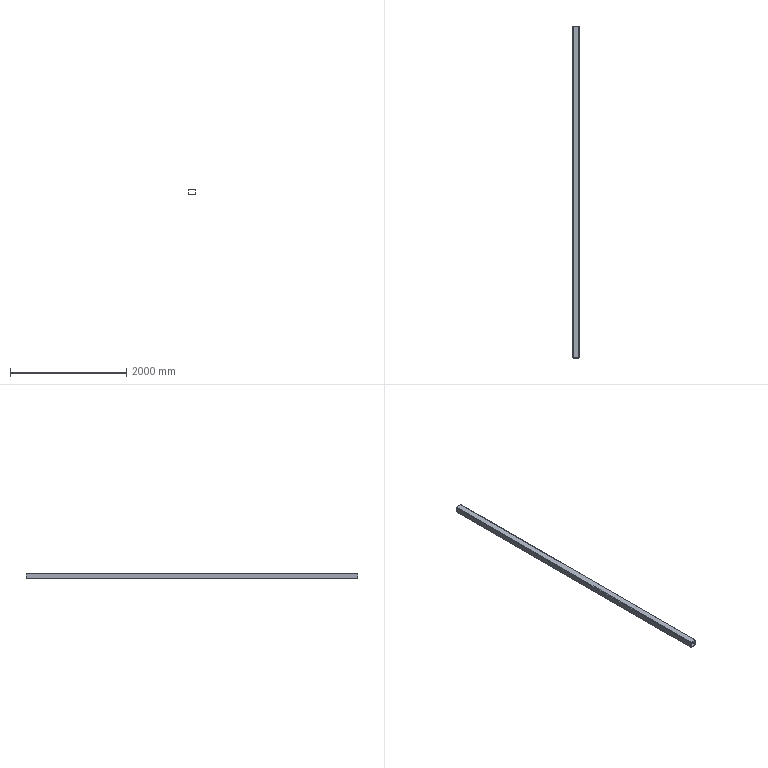Part | SolidWorks | features ExtruThin 1 | 1 solid | 18 faces | box 120 x 5702 x 100 mm | volume 9357335 mm3 | plane 10 | cylinder 8 | commonest cylinder face diameters 12 x4 20 x4
STEP:
#1=CARTESIAN_POINT('',(60.,2851.,-40.));
#2=VERTEX_POINT('',#1);
#3=CARTESIAN_POINT('',(50.,2851.,-50.));
#4=VERTEX_POINT('',#3);
#5=CARTESIAN_POINT('',(50.,2851.,-40.));
#6=DIRECTION('',(0.,1.,0.));
#7=DIRECTION('',(0.,0.,-1.));
#8=AXIS2_PLACEMENT_3D('',#5,#6,#7);
#9=CIRCLE('',#8,10.);
#10=EDGE_CURVE('',#2,#4,#9,.T.);
#11=ORIENTED_EDGE('',*,*,#10,.T.);
#12=CARTESIAN_POINT('',(-50.,2851.,-50.));
#13=VERTEX_POINT('',#12);
#14=CARTESIAN_POINT('',(-50.,2851.,-50.));
#15=DIRECTION('',(-1.,0.,0.));
#16=VECTOR('',#15,1000.);
#17=LINE('',#14,#16);
#18=EDGE_CURVE('',#4,#13,#17,.T.);
#19=ORIENTED_EDGE('',*,*,#18,.T.);
#20=CARTESIAN_POINT('',(-60.,2851.,-40.));
#21=VERTEX_POINT('',#20);
#22=CARTESIAN_POINT('',(-50.,2851.,-40.));
#23=DIRECTION('',(0.,1.,0.));
#24=DIRECTION('',(0.,0.,1.));
#25=AXIS2_PLACEMENT_3D('',#22,#23,#24);
#26=CIRCLE('',#25,10.);
#27=EDGE_CURVE('',#13,#21,#26,.T.);
#28=ORIENTED_EDGE('',*,*,#27,.T.);
#29=CARTESIAN_POINT('',(-60.,2851.,40.));
#30=VERTEX_POINT('',#29);
#31=CARTESIAN_POINT('',(-60.,2851.,-40.));
#32=DIRECTION('',(0.,0.,1.));
#33=VECTOR('',#32,1000.);
#34=LINE('',#31,#33);
#35=EDGE_CURVE('',#21,#30,#34,.T.);
#36=ORIENTED_EDGE('',*,*,#35,.T.);
#37=CARTESIAN_POINT('',(-50.,2851.,50.));
#38=VERTEX_POINT('',#37);
#39=CARTESIAN_POINT('',(-50.,2851.,40.));
#40=DIRECTION('',(0.,1.,0.));
#41=DIRECTION('',(0.,0.,1.));
#42=AXIS2_PLACEMENT_3D('',#39,#40,#41);
#43=CIRCLE('',#42,10.);
#44=EDGE_CURVE('',#30,#38,#43,.T.);
#45=ORIENTED_EDGE('',*,*,#44,.T.);
#46=CARTESIAN_POINT('',(50.,2851.,50.));
#47=VERTEX_POINT('',#46);
#48=CARTESIAN_POINT('',(-50.,2851.,50.));
#49=DIRECTION('',(1.,0.,0.));
#50=VECTOR('',#49,1000.);
#51=LINE('',#48,#50);
#52=EDGE_CURVE('',#38,#47,#51,.T.);
#53=ORIENTED_EDGE('',*,*,#52,.T.);
#54=CARTESIAN_POINT('',(60.,2851.,40.));
#55=VERTEX_POINT('',#54);
#56=CARTESIAN_POINT('',(50.,2851.,40.));
#57=DIRECTION('',(0.,1.,0.));
#58=DIRECTION('',(0.,0.,1.));
#59=AXIS2_PLACEMENT_3D('',#56,#57,#58);
#60=CIRCLE('',#59,10.);
#61=EDGE_CURVE('',#47,#55,#60,.T.);
#62=ORIENTED_EDGE('',*,*,#61,.T.);
#63=CARTESIAN_POINT('',(60.,2851.,-40.));
#64=DIRECTION('',(0.,0.,-1.));
#65=VECTOR('',#64,1000.);
#66=LINE('',#63,#65);
#67=EDGE_CURVE('',#55,#2,#66,.T.);
#68=ORIENTED_EDGE('',*,*,#67,.T.);
#69=EDGE_LOOP('',(#11,#19,#28,#36,#45,#53,#62,#68));
#70=FACE_OUTER_BOUND('',#69,.T.);
#71=CARTESIAN_POINT('',(50.,2851.,-46.));
#72=VERTEX_POINT('',#71);
#73=CARTESIAN_POINT('',(-50.,2851.,-46.));
#74=VERTEX_POINT('',#73);
#75=CARTESIAN_POINT('',(50.,2851.,-46.));
#76=DIRECTION('',(-1.,0.,0.));
#77=VECTOR('',#76,1000.);
#78=LINE('',#75,#77);
#79=EDGE_CURVE('',#72,#74,#78,.T.);
#80=ORIENTED_EDGE('',*,*,#79,.F.);
#81=CARTESIAN_POINT('',(56.,2851.,-40.));
#82=VERTEX_POINT('',#81);
#83=CARTESIAN_POINT('',(50.,2851.,-40.));
#84=DIRECTION('',(0.,1.,0.));
#85=DIRECTION('',(-1.,0.,0.));
#86=AXIS2_PLACEMENT_3D('',#83,#84,#85);
#87=CIRCLE('',#86,6.);
#88=EDGE_CURVE('',#82,#72,#87,.T.);
#89=ORIENTED_EDGE('',*,*,#88,.F.);
#90=CARTESIAN_POINT('',(56.,2851.,40.));
#91=VERTEX_POINT('',#90);
#92=CARTESIAN_POINT('',(56.,2851.,-40.));
#93=DIRECTION('',(0.,0.,-1.));
#94=VECTOR('',#93,1000.);
#95=LINE('',#92,#94);
#96=EDGE_CURVE('',#91,#82,#95,.T.);
#97=ORIENTED_EDGE('',*,*,#96,.F.);
#98=CARTESIAN_POINT('',(50.,2851.,46.));
#99=VERTEX_POINT('',#98);
#100=CARTESIAN_POINT('',(50.,2851.,40.));
#101=DIRECTION('',(0.,1.,0.));
#102=DIRECTION('',(-1.,0.,0.));
#103=AXIS2_PLACEMENT_3D('',#100,#101,#102);
#104=CIRCLE('',#103,6.);
#105=EDGE_CURVE('',#99,#91,#104,.T.);
#106=ORIENTED_EDGE('',*,*,#105,.F.);
#107=CARTESIAN_POINT('',(-50.,2851.,46.));
#108=VERTEX_POINT('',#107);
#109=CARTESIAN_POINT('',(50.,2851.,46.));
#110=DIRECTION('',(1.,0.,0.));
#111=VECTOR('',#110,1000.);
#112=LINE('',#109,#111);
#113=EDGE_CURVE('',#108,#99,#112,.T.);
#114=ORIENTED_EDGE('',*,*,#113,.F.);
#115=CARTESIAN_POINT('',(-56.,2851.,40.));
#116=VERTEX_POINT('',#115);
#117=CARTESIAN_POINT('',(-50.,2851.,40.));
#118=DIRECTION('',(0.,1.,0.));
#119=DIRECTION('',(-1.,0.,0.));
#120=AXIS2_PLACEMENT_3D('',#117,#118,#119);
#121=CIRCLE('',#120,6.);
#122=EDGE_CURVE('',#116,#108,#121,.T.);
#123=ORIENTED_EDGE('',*,*,#122,.F.);
#124=CARTESIAN_POINT('',(-56.,2851.,-40.));
#125=VERTEX_POINT('',#124);
#126=CARTESIAN_POINT('',(-56.,2851.,-40.));
#127=DIRECTION('',(0.,0.,1.));
#128=VECTOR('',#127,1000.);
#129=LINE('',#126,#128);
#130=EDGE_CURVE('',#125,#116,#129,.T.);
#131=ORIENTED_EDGE('',*,*,#130,.F.);
#132=CARTESIAN_POINT('',(-50.,2851.,-40.));
#133=DIRECTION('',(0.,1.,0.));
#134=DIRECTION('',(-1.,0.,0.));
#135=AXIS2_PLACEMENT_3D('',#132,#133,#134);
#136=CIRCLE('',#135,6.);
#137=EDGE_CURVE('',#74,#125,#136,.T.);
#138=ORIENTED_EDGE('',*,*,#137,.F.);
#139=EDGE_LOOP('',(#80,#89,#97,#106,#114,#123,#131,#138));
#140=FACE_BOUND('',#139,.T.);
#141=CARTESIAN_POINT('',(50.,2851.,-40.));
#142=DIRECTION('',(0.,1.,0.));
#143=DIRECTION('',(0.,0.,1.));
#144=AXIS2_PLACEMENT_3D('',#141,#142,#143);
#145=PLANE('',#144);
#146=ADVANCED_FACE('',(#70,#140),#145,.T.);
#147=CARTESIAN_POINT('',(60.,-2851.,-40.));
#148=VERTEX_POINT('',#147);
#149=CARTESIAN_POINT('',(50.,-2851.,-50.));
#150=VERTEX_POINT('',#149);
#151=CARTESIAN_POINT('',(50.,-2851.,-40.));
#152=DIRECTION('',(0.,1.,0.));
#153=DIRECTION('',(0.,0.,-1.));
#154=AXIS2_PLACEMENT_3D('',#151,#152,#153);
#155=CIRCLE('',#154,10.);
#156=EDGE_CURVE('',#148,#150,#155,.T.);
#157=ORIENTED_EDGE('',*,*,#156,.F.);
#158=CARTESIAN_POINT('',(60.,-2851.,40.));
#159=VERTEX_POINT('',#158);
#160=CARTESIAN_POINT('',(60.,-2851.,-40.));
#161=DIRECTION('',(0.,0.,-1.));
#162=VECTOR('',#161,1000.);
#163=LINE('',#160,#162);
#164=EDGE_CURVE('',#159,#148,#163,.T.);
#165=ORIENTED_EDGE('',*,*,#164,.F.);
#166=CARTESIAN_POINT('',(50.,-2851.,50.));
#167=VERTEX_POINT('',#166);
#168=CARTESIAN_POINT('',(50.,-2851.,40.));
#169=DIRECTION('',(0.,1.,0.));
#170=DIRECTION('',(0.,0.,1.));
#171=AXIS2_PLACEMENT_3D('',#168,#169,#170);
#172=CIRCLE('',#171,10.);
#173=EDGE_CURVE('',#167,#159,#172,.T.);
#174=ORIENTED_EDGE('',*,*,#173,.F.);
#175=CARTESIAN_POINT('',(-50.,-2851.,50.));
#176=VERTEX_POINT('',#175);
#177=CARTESIAN_POINT('',(-50.,-2851.,50.));
#178=DIRECTION('',(1.,0.,0.));
#179=VECTOR('',#178,1000.);
#180=LINE('',#177,#179);
#181=EDGE_CURVE('',#176,#167,#180,.T.);
#182=ORIENTED_EDGE('',*,*,#181,.F.);
#183=CARTESIAN_POINT('',(-60.,-2851.,40.));
#184=VERTEX_POINT('',#183);
#185=CARTESIAN_POINT('',(-50.,-2851.,40.));
#186=DIRECTION('',(0.,1.,0.));
#187=DIRECTION('',(0.,0.,1.));
#188=AXIS2_PLACEMENT_3D('',#185,#186,#187);
#189=CIRCLE('',#188,10.);
#190=EDGE_CURVE('',#184,#176,#189,.T.);
#191=ORIENTED_EDGE('',*,*,#190,.F.);
#192=CARTESIAN_POINT('',(-60.,-2851.,-40.));
#193=VERTEX_POINT('',#192);
#194=CARTESIAN_POINT('',(-60.,-2851.,-40.));
#195=DIRECTION('',(0.,0.,1.));
#196=VECTOR('',#195,1000.);
#197=LINE('',#194,#196);
#198=EDGE_CURVE('',#193,#184,#197,.T.);
#199=ORIENTED_EDGE('',*,*,#198,.F.);
#200=CARTESIAN_POINT('',(-50.,-2851.,-50.));
#201=VERTEX_POINT('',#200);
#202=CARTESIAN_POINT('',(-50.,-2851.,-40.));
#203=DIRECTION('',(0.,1.,0.));
#204=DIRECTION('',(0.,0.,1.));
#205=AXIS2_PLACEMENT_3D('',#202,#203,#204);
#206=CIRCLE('',#205,10.);
#207=EDGE_CURVE('',#201,#193,#206,.T.);
#208=ORIENTED_EDGE('',*,*,#207,.F.);
#209=CARTESIAN_POINT('',(-50.,-2851.,-50.));
#210=DIRECTION('',(-1.,0.,0.));
#211=VECTOR('',#210,1000.);
#212=LINE('',#209,#211);
#213=EDGE_CURVE('',#150,#201,#212,.T.);
#214=ORIENTED_EDGE('',*,*,#213,.F.);
#215=EDGE_LOOP('',(#157,#165,#174,#182,#191,#199,#208,#214));
#216=FACE_OUTER_BOUND('',#215,.T.);
#217=CARTESIAN_POINT('',(56.,-2851.,-40.));
#218=VERTEX_POINT('',#217);
#219=CARTESIAN_POINT('',(50.,-2851.,-46.));
#220=VERTEX_POINT('',#219);
#221=CARTESIAN_POINT('',(50.,-2851.,-40.));
#222=DIRECTION('',(0.,1.,0.));
#223=DIRECTION('',(-1.,0.,0.));
#224=AXIS2_PLACEMENT_3D('',#221,#222,#223);
#225=CIRCLE('',#224,6.);
#226=EDGE_CURVE('',#218,#220,#225,.T.);
#227=ORIENTED_EDGE('',*,*,#226,.T.);
#228=CARTESIAN_POINT('',(-50.,-2851.,-46.));
#229=VERTEX_POINT('',#228);
#230=CARTESIAN_POINT('',(50.,-2851.,-46.));
#231=DIRECTION('',(-1.,0.,0.));
#232=VECTOR('',#231,1000.);
#233=LINE('',#230,#232);
#234=EDGE_CURVE('',#220,#229,#233,.T.);
#235=ORIENTED_EDGE('',*,*,#234,.T.);
#236=CARTESIAN_POINT('',(-56.,-2851.,-40.));
#237=VERTEX_POINT('',#236);
#238=CARTESIAN_POINT('',(-50.,-2851.,-40.));
#239=DIRECTION('',(0.,1.,0.));
#240=DIRECTION('',(-1.,0.,0.));
#241=AXIS2_PLACEMENT_3D('',#238,#239,#240);
#242=CIRCLE('',#241,6.);
#243=EDGE_CURVE('',#229,#237,#242,.T.);
#244=ORIENTED_EDGE('',*,*,#243,.T.);
#245=CARTESIAN_POINT('',(-56.,-2851.,40.));
#246=VERTEX_POINT('',#245);
#247=CARTESIAN_POINT('',(-56.,-2851.,-40.));
#248=DIRECTION('',(0.,0.,1.));
#249=VECTOR('',#248,1000.);
#250=LINE('',#247,#249);
#251=EDGE_CURVE('',#237,#246,#250,.T.);
#252=ORIENTED_EDGE('',*,*,#251,.T.);
#253=CARTESIAN_POINT('',(-50.,-2851.,46.));
#254=VERTEX_POINT('',#253);
#255=CARTESIAN_POINT('',(-50.,-2851.,40.));
#256=DIRECTION('',(0.,1.,0.));
#257=DIRECTION('',(-1.,0.,0.));
#258=AXIS2_PLACEMENT_3D('',#255,#256,#257);
#259=CIRCLE('',#258,6.);
#260=EDGE_CURVE('',#246,#254,#259,.T.);
#261=ORIENTED_EDGE('',*,*,#260,.T.);
#262=CARTESIAN_POINT('',(50.,-2851.,46.));
#263=VERTEX_POINT('',#262);
#264=CARTESIAN_POINT('',(50.,-2851.,46.));
#265=DIRECTION('',(1.,0.,0.));
#266=VECTOR('',#265,1000.);
#267=LINE('',#264,#266);
#268=EDGE_CURVE('',#254,#263,#267,.T.);
#269=ORIENTED_EDGE('',*,*,#268,.T.);
#270=CARTESIAN_POINT('',(56.,-2851.,40.));
#271=VERTEX_POINT('',#270);
#272=CARTESIAN_POINT('',(50.,-2851.,40.));
#273=DIRECTION('',(0.,1.,0.));
#274=DIRECTION('',(-1.,0.,0.));
#275=AXIS2_PLACEMENT_3D('',#272,#273,#274);
#276=CIRCLE('',#275,6.);
#277=EDGE_CURVE('',#263,#271,#276,.T.);
#278=ORIENTED_EDGE('',*,*,#277,.T.);
#279=CARTESIAN_POINT('',(56.,-2851.,-40.));
#280=DIRECTION('',(0.,0.,-1.));
#281=VECTOR('',#280,1000.);
#282=LINE('',#279,#281);
#283=EDGE_CURVE('',#271,#218,#282,.T.);
#284=ORIENTED_EDGE('',*,*,#283,.T.);
#285=EDGE_LOOP('',(#227,#235,#244,#252,#261,#269,#278,#284));
#286=FACE_BOUND('',#285,.T.);
#287=CARTESIAN_POINT('',(50.,-2851.,-40.));
#288=DIRECTION('',(0.,1.,0.));
#289=DIRECTION('',(0.,0.,1.));
#290=AXIS2_PLACEMENT_3D('',#287,#288,#289);
#291=PLANE('',#290);
#292=ADVANCED_FACE('',(#216,#286),#291,.F.);
#293=ORIENTED_EDGE('',*,*,#156,.T.);
#294=CARTESIAN_POINT('',(50.,2851.,-50.));
#295=DIRECTION('',(0.,-1.,0.));
#296=VECTOR('',#295,1000.);
#297=LINE('',#294,#296);
#298=EDGE_CURVE('',#4,#150,#297,.T.);
#299=ORIENTED_EDGE('',*,*,#298,.F.);
#300=ORIENTED_EDGE('',*,*,#10,.F.);
#301=CARTESIAN_POINT('',(60.,2851.,-40.));
#302=DIRECTION('',(0.,-1.,0.));
#303=VECTOR('',#302,1000.);
#304=LINE('',#301,#303);
#305=EDGE_CURVE('',#2,#148,#304,.T.);
#306=ORIENTED_EDGE('',*,*,#305,.T.);
#307=EDGE_LOOP('',(#293,#299,#300,#306));
#308=FACE_OUTER_BOUND('',#307,.T.);
#309=CARTESIAN_POINT('',(50.,2851.,-40.));
#310=DIRECTION('',(0.,-1.,0.));
#311=DIRECTION('',(0.,0.,-1.));
#312=AXIS2_PLACEMENT_3D('',#309,#310,#311);
#313=CYLINDRICAL_SURFACE('',#312,10.);
#314=ADVANCED_FACE('',(#308),#313,.T.);
#315=ORIENTED_EDGE('',*,*,#213,.T.);
#316=CARTESIAN_POINT('',(-50.,2851.,-50.));
#317=DIRECTION('',(0.,-1.,0.));
#318=VECTOR('',#317,1000.);
#319=LINE('',#316,#318);
#320=EDGE_CURVE('',#13,#201,#319,.T.);
#321=ORIENTED_EDGE('',*,*,#320,.F.);
#322=ORIENTED_EDGE('',*,*,#18,.F.);
#323=ORIENTED_EDGE('',*,*,#298,.T.);
#324=EDGE_LOOP('',(#315,#321,#322,#323));
#325=FACE_OUTER_BOUND('',#324,.T.);
#326=CARTESIAN_POINT('',(-50.,2851.,-50.));
#327=DIRECTION('',(0.,0.,1.));
#328=DIRECTION('',(1.,0.,0.));
#329=AXIS2_PLACEMENT_3D('',#326,#327,#328);
#330=PLANE('',#329);
#331=ADVANCED_FACE('',(#325),#330,.F.);
#332=ORIENTED_EDGE('',*,*,#207,.T.);
#333=CARTESIAN_POINT('',(-60.,2851.,-40.));
#334=DIRECTION('',(0.,-1.,0.));
#335=VECTOR('',#334,1000.);
#336=LINE('',#333,#335);
#337=EDGE_CURVE('',#21,#193,#336,.T.);
#338=ORIENTED_EDGE('',*,*,#337,.F.);
#339=ORIENTED_EDGE('',*,*,#27,.F.);
#340=ORIENTED_EDGE('',*,*,#320,.T.);
#341=EDGE_LOOP('',(#332,#338,#339,#340));
#342=FACE_OUTER_BOUND('',#341,.T.);
#343=CARTESIAN_POINT('',(-50.,2851.,-40.));
#344=DIRECTION('',(0.,-1.,0.));
#345=DIRECTION('',(0.,0.,-1.));
#346=AXIS2_PLACEMENT_3D('',#343,#344,#345);
#347=CYLINDRICAL_SURFACE('',#346,10.);
#348=ADVANCED_FACE('',(#342),#347,.T.);
#349=ORIENTED_EDGE('',*,*,#198,.T.);
#350=CARTESIAN_POINT('',(-60.,2851.,40.));
#351=DIRECTION('',(0.,-1.,0.));
#352=VECTOR('',#351,1000.);
#353=LINE('',#350,#352);
#354=EDGE_CURVE('',#30,#184,#353,.T.);
#355=ORIENTED_EDGE('',*,*,#354,.F.);
#356=ORIENTED_EDGE('',*,*,#35,.F.);
#357=ORIENTED_EDGE('',*,*,#337,.T.);
#358=EDGE_LOOP('',(#349,#355,#356,#357));
#359=FACE_OUTER_BOUND('',#358,.T.);
#360=CARTESIAN_POINT('',(-60.,2851.,-40.));
#361=DIRECTION('',(1.,0.,0.));
#362=DIRECTION('',(0.,0.,-1.));
#363=AXIS2_PLACEMENT_3D('',#360,#361,#362);
#364=PLANE('',#363);
#365=ADVANCED_FACE('',(#359),#364,.F.);
#366=ORIENTED_EDGE('',*,*,#190,.T.);
#367=CARTESIAN_POINT('',(-50.,2851.,50.));
#368=DIRECTION('',(0.,-1.,0.));
#369=VECTOR('',#368,1000.);
#370=LINE('',#367,#369);
#371=EDGE_CURVE('',#38,#176,#370,.T.);
#372=ORIENTED_EDGE('',*,*,#371,.F.);
#373=ORIENTED_EDGE('',*,*,#44,.F.);
#374=ORIENTED_EDGE('',*,*,#354,.T.);
#375=EDGE_LOOP('',(#366,#372,#373,#374));
#376=FACE_OUTER_BOUND('',#375,.T.);
#377=CARTESIAN_POINT('',(-50.,2851.,40.));
#378=DIRECTION('',(0.,-1.,0.));
#379=DIRECTION('',(0.,0.,-1.));
#380=AXIS2_PLACEMENT_3D('',#377,#378,#379);
#381=CYLINDRICAL_SURFACE('',#380,10.);
#382=ADVANCED_FACE('',(#376),#381,.T.);
#383=ORIENTED_EDGE('',*,*,#181,.T.);
#384=CARTESIAN_POINT('',(50.,2851.,50.));
#385=DIRECTION('',(0.,-1.,0.));
#386=VECTOR('',#385,1000.);
#387=LINE('',#384,#386);
#388=EDGE_CURVE('',#47,#167,#387,.T.);
#389=ORIENTED_EDGE('',*,*,#388,.F.);
#390=ORIENTED_EDGE('',*,*,#52,.F.);
#391=ORIENTED_EDGE('',*,*,#371,.T.);
#392=EDGE_LOOP('',(#383,#389,#390,#391));
#393=FACE_OUTER_BOUND('',#392,.T.);
#394=CARTESIAN_POINT('',(-50.,2851.,50.));
#395=DIRECTION('',(0.,0.,-1.));
#396=DIRECTION('',(-1.,0.,0.));
#397=AXIS2_PLACEMENT_3D('',#394,#395,#396);
#398=PLANE('',#397);
#399=ADVANCED_FACE('',(#393),#398,.F.);
#400=ORIENTED_EDGE('',*,*,#173,.T.);
#401=CARTESIAN_POINT('',(60.,2851.,40.));
#402=DIRECTION('',(0.,-1.,0.));
#403=VECTOR('',#402,1000.);
#404=LINE('',#401,#403);
#405=EDGE_CURVE('',#55,#159,#404,.T.);
#406=ORIENTED_EDGE('',*,*,#405,.F.);
#407=ORIENTED_EDGE('',*,*,#61,.F.);
#408=ORIENTED_EDGE('',*,*,#388,.T.);
#409=EDGE_LOOP('',(#400,#406,#407,#408));
#410=FACE_OUTER_BOUND('',#409,.T.);
#411=CARTESIAN_POINT('',(50.,2851.,40.));
#412=DIRECTION('',(0.,-1.,0.));
#413=DIRECTION('',(0.,0.,-1.));
#414=AXIS2_PLACEMENT_3D('',#411,#412,#413);
#415=CYLINDRICAL_SURFACE('',#414,10.);
#416=ADVANCED_FACE('',(#410),#415,.T.);
#417=ORIENTED_EDGE('',*,*,#164,.T.);
#418=ORIENTED_EDGE('',*,*,#305,.F.);
#419=ORIENTED_EDGE('',*,*,#67,.F.);
#420=ORIENTED_EDGE('',*,*,#405,.T.);
#421=EDGE_LOOP('',(#417,#418,#419,#420));
#422=FACE_OUTER_BOUND('',#421,.T.);
#423=CARTESIAN_POINT('',(60.,2851.,-40.));
#424=DIRECTION('',(-1.,0.,0.));
#425=DIRECTION('',(0.,0.,1.));
#426=AXIS2_PLACEMENT_3D('',#423,#424,#425);
#427=PLANE('',#426);
#428=ADVANCED_FACE('',(#422),#427,.F.);
#429=ORIENTED_EDGE('',*,*,#226,.F.);
#430=CARTESIAN_POINT('',(56.,2851.,-40.));
#431=DIRECTION('',(0.,-1.,0.));
#432=VECTOR('',#431,1000.);
#433=LINE('',#430,#432);
#434=EDGE_CURVE('',#82,#218,#433,.T.);
#435=ORIENTED_EDGE('',*,*,#434,.F.);
#436=ORIENTED_EDGE('',*,*,#88,.T.);
#437=CARTESIAN_POINT('',(50.,2851.,-46.));
#438=DIRECTION('',(0.,-1.,0.));
#439=VECTOR('',#438,1000.);
#440=LINE('',#437,#439);
#441=EDGE_CURVE('',#72,#220,#440,.T.);
#442=ORIENTED_EDGE('',*,*,#441,.T.);
#443=EDGE_LOOP('',(#429,#435,#436,#442));
#444=FACE_OUTER_BOUND('',#443,.T.);
#445=CARTESIAN_POINT('',(50.,2851.,-40.));
#446=DIRECTION('',(0.,-1.,0.));
#447=DIRECTION('',(0.,0.,-1.));
#448=AXIS2_PLACEMENT_3D('',#445,#446,#447);
#449=CYLINDRICAL_SURFACE('',#448,6.);
#450=ADVANCED_FACE('',(#444),#449,.F.);
#451=ORIENTED_EDGE('',*,*,#234,.F.);
#452=ORIENTED_EDGE('',*,*,#441,.F.);
#453=ORIENTED_EDGE('',*,*,#79,.T.);
#454=CARTESIAN_POINT('',(-50.,2851.,-46.));
#455=DIRECTION('',(0.,-1.,0.));
#456=VECTOR('',#455,1000.);
#457=LINE('',#454,#456);
#458=EDGE_CURVE('',#74,#229,#457,.T.);
#459=ORIENTED_EDGE('',*,*,#458,.T.);
#460=EDGE_LOOP('',(#451,#452,#453,#459));
#461=FACE_OUTER_BOUND('',#460,.T.);
#462=CARTESIAN_POINT('',(50.,2851.,-46.));
#463=DIRECTION('',(0.,0.,1.));
#464=DIRECTION('',(1.,0.,0.));
#465=AXIS2_PLACEMENT_3D('',#462,#463,#464);
#466=PLANE('',#465);
#467=ADVANCED_FACE('',(#461),#466,.T.);
#468=ORIENTED_EDGE('',*,*,#243,.F.);
#469=ORIENTED_EDGE('',*,*,#458,.F.);
#470=ORIENTED_EDGE('',*,*,#137,.T.);
#471=CARTESIAN_POINT('',(-56.,2851.,-40.));
#472=DIRECTION('',(0.,-1.,0.));
#473=VECTOR('',#472,1000.);
#474=LINE('',#471,#473);
#475=EDGE_CURVE('',#125,#237,#474,.T.);
#476=ORIENTED_EDGE('',*,*,#475,.T.);
#477=EDGE_LOOP('',(#468,#469,#470,#476));
#478=FACE_OUTER_BOUND('',#477,.T.);
#479=CARTESIAN_POINT('',(-50.,2851.,-40.));
#480=DIRECTION('',(0.,-1.,0.));
#481=DIRECTION('',(0.,0.,-1.));
#482=AXIS2_PLACEMENT_3D('',#479,#480,#481);
#483=CYLINDRICAL_SURFACE('',#482,6.);
#484=ADVANCED_FACE('',(#478),#483,.F.);
#485=ORIENTED_EDGE('',*,*,#251,.F.);
#486=ORIENTED_EDGE('',*,*,#475,.F.);
#487=ORIENTED_EDGE('',*,*,#130,.T.);
#488=CARTESIAN_POINT('',(-56.,2851.,40.));
#489=DIRECTION('',(0.,-1.,0.));
#490=VECTOR('',#489,1000.);
#491=LINE('',#488,#490);
#492=EDGE_CURVE('',#116,#246,#491,.T.);
#493=ORIENTED_EDGE('',*,*,#492,.T.);
#494=EDGE_LOOP('',(#485,#486,#487,#493));
#495=FACE_OUTER_BOUND('',#494,.T.);
#496=CARTESIAN_POINT('',(-56.,2851.,-40.));
#497=DIRECTION('',(1.,0.,0.));
#498=DIRECTION('',(0.,0.,-1.));
#499=AXIS2_PLACEMENT_3D('',#496,#497,#498);
#500=PLANE('',#499);
#501=ADVANCED_FACE('',(#495),#500,.T.);
#502=ORIENTED_EDGE('',*,*,#260,.F.);
#503=ORIENTED_EDGE('',*,*,#492,.F.);
#504=ORIENTED_EDGE('',*,*,#122,.T.);
#505=CARTESIAN_POINT('',(-50.,2851.,46.));
#506=DIRECTION('',(0.,-1.,0.));
#507=VECTOR('',#506,1000.);
#508=LINE('',#505,#507);
#509=EDGE_CURVE('',#108,#254,#508,.T.);
#510=ORIENTED_EDGE('',*,*,#509,.T.);
#511=EDGE_LOOP('',(#502,#503,#504,#510));
#512=FACE_OUTER_BOUND('',#511,.T.);
#513=CARTESIAN_POINT('',(-50.,2851.,40.));
#514=DIRECTION('',(0.,-1.,0.));
#515=DIRECTION('',(0.,0.,-1.));
#516=AXIS2_PLACEMENT_3D('',#513,#514,#515);
#517=CYLINDRICAL_SURFACE('',#516,6.);
#518=ADVANCED_FACE('',(#512),#517,.F.);
#519=ORIENTED_EDGE('',*,*,#268,.F.);
#520=ORIENTED_EDGE('',*,*,#509,.F.);
#521=ORIENTED_EDGE('',*,*,#113,.T.);
#522=CARTESIAN_POINT('',(50.,2851.,46.));
#523=DIRECTION('',(0.,-1.,0.));
#524=VECTOR('',#523,1000.);
#525=LINE('',#522,#524);
#526=EDGE_CURVE('',#99,#263,#525,.T.);
#527=ORIENTED_EDGE('',*,*,#526,.T.);
#528=EDGE_LOOP('',(#519,#520,#521,#527));
#529=FACE_OUTER_BOUND('',#528,.T.);
#530=CARTESIAN_POINT('',(50.,2851.,46.));
#531=DIRECTION('',(0.,0.,-1.));
#532=DIRECTION('',(-1.,0.,0.));
#533=AXIS2_PLACEMENT_3D('',#530,#531,#532);
#534=PLANE('',#533);
#535=ADVANCED_FACE('',(#529),#534,.T.);
#536=ORIENTED_EDGE('',*,*,#277,.F.);
#537=ORIENTED_EDGE('',*,*,#526,.F.);
#538=ORIENTED_EDGE('',*,*,#105,.T.);
#539=CARTESIAN_POINT('',(56.,2851.,40.));
#540=DIRECTION('',(0.,-1.,0.));
#541=VECTOR('',#540,1000.);
#542=LINE('',#539,#541);
#543=EDGE_CURVE('',#91,#271,#542,.T.);
#544=ORIENTED_EDGE('',*,*,#543,.T.);
#545=EDGE_LOOP('',(#536,#537,#538,#544));
#546=FACE_OUTER_BOUND('',#545,.T.);
#547=CARTESIAN_POINT('',(50.,2851.,40.));
#548=DIRECTION('',(0.,-1.,0.));
#549=DIRECTION('',(0.,0.,-1.));
#550=AXIS2_PLACEMENT_3D('',#547,#548,#549);
#551=CYLINDRICAL_SURFACE('',#550,6.);
#552=ADVANCED_FACE('',(#546),#551,.F.);
#553=ORIENTED_EDGE('',*,*,#283,.F.);
#554=ORIENTED_EDGE('',*,*,#543,.F.);
#555=ORIENTED_EDGE('',*,*,#96,.T.);
#556=ORIENTED_EDGE('',*,*,#434,.T.);
#557=EDGE_LOOP('',(#553,#554,#555,#556));
#558=FACE_OUTER_BOUND('',#557,.T.);
#559=CARTESIAN_POINT('',(56.,2851.,-40.));
#560=DIRECTION('',(-1.,0.,0.));
#561=DIRECTION('',(0.,0.,1.));
#562=AXIS2_PLACEMENT_3D('',#559,#560,#561);
#563=PLANE('',#562);
#564=ADVANCED_FACE('',(#558),#563,.T.);
#565=CLOSED_SHELL('',(#146,#292,#314,#331,#348,#365,#382,#399,#416,#428,#450,#467,#484,#501,#518,#535,#552,#564));
#566=MANIFOLD_SOLID_BREP('',#565);
#567=CARTESIAN_POINT('',(0.,0.,0.));
#568=DIRECTION('',(0.,0.,1.));
#569=DIRECTION('',(1.,0.,0.));
#570=AXIS2_PLACEMENT_3D('',#567,#568,#569);
#571=(LENGTH_UNIT()NAMED_UNIT(*)SI_UNIT(.MILLI.,.METRE.));
#572=UNCERTAINTY_MEASURE_WITH_UNIT(LENGTH_MEASURE(0.00001),#571,'','');
#573=(NAMED_UNIT(*)PLANE_ANGLE_UNIT()SI_UNIT($,.RADIAN.));
#574=(NAMED_UNIT(*)SI_UNIT($,.STERADIAN.)SOLID_ANGLE_UNIT());
#575=(GEOMETRIC_REPRESENTATION_CONTEXT(3)GLOBAL_UNCERTAINTY_ASSIGNED_CONTEXT((#572))GLOBAL_UNIT_ASSIGNED_CONTEXT((#571,#573,#574))REPRESENTATION_CONTEXT('',''));
#576=ADVANCED_BREP_SHAPE_REPRESENTATION('',(#566,#570),#575);